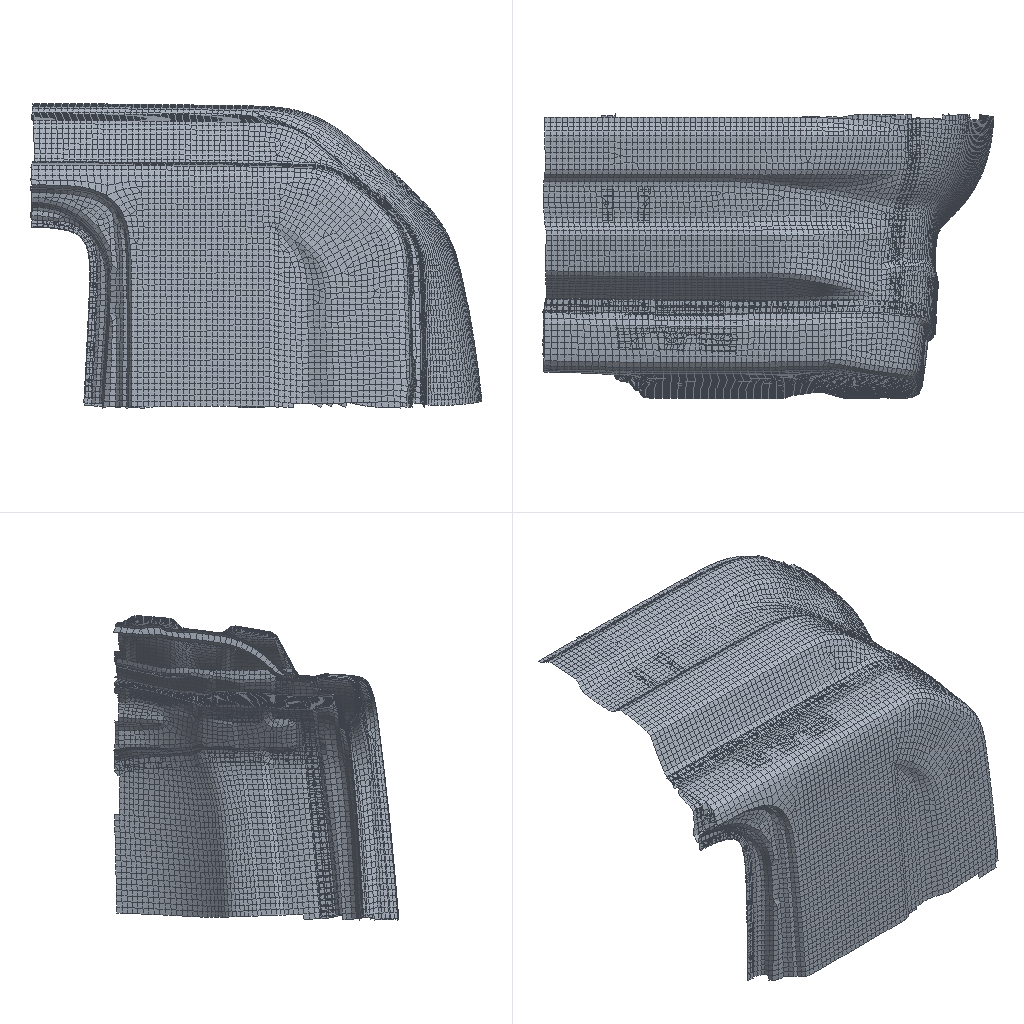Simulation study | nastran
Set-up summary:
category,name,step,type,value,unit,region
solver,nx_nastran
units,not stated in the deck,,not stated
analysis,deck,,static,static
analysis,solution,,SOL,101
load_step,SUBCASE 2,2,SUBCASE,SPC=2 LOAD=3
load_step,SUBCASE 3,3,SUBCASE,SPC=2 LOAD=4
load_step,SUBCASE 4,4,SUBCASE,SPC=2 LOAD=5
load_step,requested,,,3
mesh,nodes,,,15964
mesh,elements,,,14750
element_type,CHEXA,,unverified,89
element_type,CQUAD4,,shell,14349
element_type,CTRIA3,,shell,401
load,load commands in deck,,count,3
bc,support commands in deck,,count,339
check,setup vs results,,match,"every grid point's frame and coordinates and every element id; grid points of CHEXA, CQUAD4, CTRIA3 elements"
Nastran input file, long lists of numbers shortened:
$$------------------------------------------------------------------------------$
$$                                                                              $
$$ NASTRAN Input Deck Generated by HyperMesh Version  :10.0buil                 $
$$ Generated using HyperMesh-Nastran Template Version : 10.0build60
$$                                                                              $
$$   Template:  general                                                         $
$$                                                                              $
$$------------------------------------------------------------------------------$
$$------------------------------------------------------------------------------$
$$                      Executive Control Cards                                 $
$$------------------------------------------------------------------------------$
SOL 101
CEND
$$------------------------------------------------------------------------------$
$$                      Case Control Cards                                      $
$$------------------------------------------------------------------------------$
  DISPLACEMENT = ALL
  ESE = ALL
$
$HMNAME LOADSTEP               2"fx"
SUBCASE       2
  LABEL=  fx
  SPC =        2
  LOAD =        3
$
$HMNAME LOADSTEP               3"fy"
SUBCASE       3
  LABEL=  fy
  SPC =        2
  LOAD =        4
$
$HMNAME LOADSTEP               4"fz"
SUBCASE       4
  LABEL=  fz
  SPC =        2
  LOAD =        5
$$------------------------------------------------------------------------------$
$$                      Bulk Data Cards                                         $
$$------------------------------------------------------------------------------$
BEGIN BULK
PARAM,POST,-1
$$
$$  GRID Data
$$
GRID       36894        283.9736-826.0441700.04
GRID       36895        284.1967-815.43 1701.44
$ (15962 more lines like these left out)
$$
$$  SPOINT Data
$$
$$
$$------------------------------------------------------------------------------$
$$             Group Definitions                                                $
$$------------------------------------------------------------------------------$
$$
$$ RBE2 Elements - Multiple dependent nodes
$$
RBE2     101299884098465  1234565400408454004154540042535400433854004397+
+       5400442754004442540044725400448654004531540045345400477154004889+
+       5400515354005290540053515400535254005479540054935400549754005504+
+       5400550654005529540055305400553354005534540055405400554154005542+
+       5400628054006287540064765400648454006489540064935400649954006505+
+       5400651054006517540072485400727554007282540072835400759554007596+
+       5400827254008290540082925400830354008307540098355400992454010999+
+       5401100154011017540110195401103554011037540110545401105554011073+
+       5401107454011092540110935401111154011112540111305401113154011149+
+       5401115054011167540111695401118554011187540112035401120554011221+
+       5401122354011239540112415401125754011259540112765401127754011294+
+       5401129554011313540119805401198154012059540120605401206154012062+
+       5401232154012352540123535401355854013581540135885401359154013644+
+       5401364854013711540137235401378354013784540138675401418454014210+
+       5401421154014252540142835401432854014364540143795403043854030439+
+       5403045054030451540305065403051354030522540305245403053254030533+
+       5403054354030544540305475403055154030555540305585403056354030567+
+       5403057354030611540306325403102054031021540310305403104754031051+
+       5403105354031055540310565403105854031060540310615403106254031065+
+       5403111754031176540311775403130054031301540313025403130354031304+
+       5403132554031328540313295403133254031335540313385403139154031392+
+       5403139354031394540314075403141454031418540314235403142654031431+
+       5403143254031433540314355403143654031455540314605403146454031465+
+       5403147054031471540314725403147754031490540314915403149454031495+
+       5403149754031637540318475403187554031882540318945403236154032397+
+       5403239854032415540324175403241954032446540324905403249754032540+
+       5403254754032580540336455403364654033650540336565403365854033659+
+       54033662540336725403367754033680
$
$HMMOVE 84022688
$        1012998
$
$
$  RBE3 Elements
$
RBE3      997679        84084197  1234560.094908     123540701290.363805+
+            123540701250.429295     123540701280.111992     12354070132
RBE3      997680        84084198  1234560.01023      123540701260.035144+
+            123540344590.73939      123540701250.215235     12354070129
$ (1356 more lines like these left out)
$
$HMMOVE 84022687
$         997679THRU      997682  997684THRU      997691  997693THRU      997700
$         997702THRU      997709  997711THRU      997718  997720THRU      997727
$ (38 more lines like these left out)
CTRIA3    631410       1540044985400448954004504
CTRIA3    631554       1540044925400531654004404
$ (399 more lines like these left out)
$
$HMMOVE 54001010
$         631410  631554  631913  631929  631940  631942  631947THRU      631949
$         631953  631955  631968THRU      631969  631971  631975  631979  631983
$ (74 more lines like these left out)
CQUAD4      7714       154004779540044975400450554004132
CQUAD4      7715       154004483540044965400425054004524
$ (14347 more lines like these left out)
$
$HMMOVE 54001010
$           7714THRU        7716   16708   16710   16712THRU       16721   16723
$       THRU       16725   16728THRU       16730   16735THRU       16736   16743
$ (454 more lines like these left out)
CHEXA     990264      1284059017840590288405904784058913   36899   36913+
+          36901   36900
CHEXA     990265      1284059028840590338405903984059047   36913   36895+
+          36902   36901
$ (174 more lines like these left out)
$
$HMMOVE       16
$         990264THRU      990267
$
$ (77 more lines like these left out)
PSHELL         1       10.8            1               1
$
$HMNAME PROP                   4"150T" 4
$HWCOLOR PROP                  4       6
PSHELL         4       11.5            1               1
$
$HMNAME PROP                   9"70T" 4
$HWCOLOR PROP                  9      17
PSHELL         9       10.7            1               1
$$
$$  PSOLID Data
$
$HMNAME PROP                  12"glue" 5
$HWCOLOR PROP                 12      21
PSOLID        12       8
$
$HMNAME PROP                  15"spot" 5
$HWCOLOR PROP                 15      24
PSOLID        15       1
$$
$$------------------------------------------------------------------------------$
$$                      Material Definition Cards                               $
$$------------------------------------------------------------------------------$
$$--------------------------------------------------------------
$$ HYPERMESH TAGS
$$--------------------------------------------------------------
$$BEGIN TAGS
$$END TAGS
$$
$$  MAT1 Data
$
$HMNAME MAT                    1"steel" "MAT1"
$HWCOLOR MAT                   1       3
MAT1           1210000.0        0.3     7.90E-09
$
$HMNAME MAT                    8"glue" "MAT1"
$HWCOLOR MAT                   8       4
MAT1           8400.0           0.4     1.00E-10
$$
$$
$$
$$------------------------------------------------------------------------------$
$ (42 more lines like these left out)
SPC            2   37802  1234560.0
SPC            2   37815  1234560.0
SPC            2   37823  1234560.0
SPC            2   37851  1234560.0
$ (335 more lines like these left out)
$$
$$  FORCE Data
$$
FORCE          384098465       01.0     500.0   0.0     0.0
FORCE          484098465       01.0     0.0     500.0   0.0
FORCE          584098465       01.0     0.0     0.0     500.0
$HMASSEM 5400010       4 5400010
$HMASSEM_IDS    54001010540050105400511054005310
$HMASSEM 5600101       6 5600010
$HMASSEM_IDS    5600101056001020
$HMASSEM 5700010       8 5700010
$HMASSEM_IDS    5700101057001030      16
$
ENDDATA
Results summary:
result,analysis,,,static
result,last_loadstep,,,3
result,primary field,,,displacements
result,max displacement,,,0.7187,model units